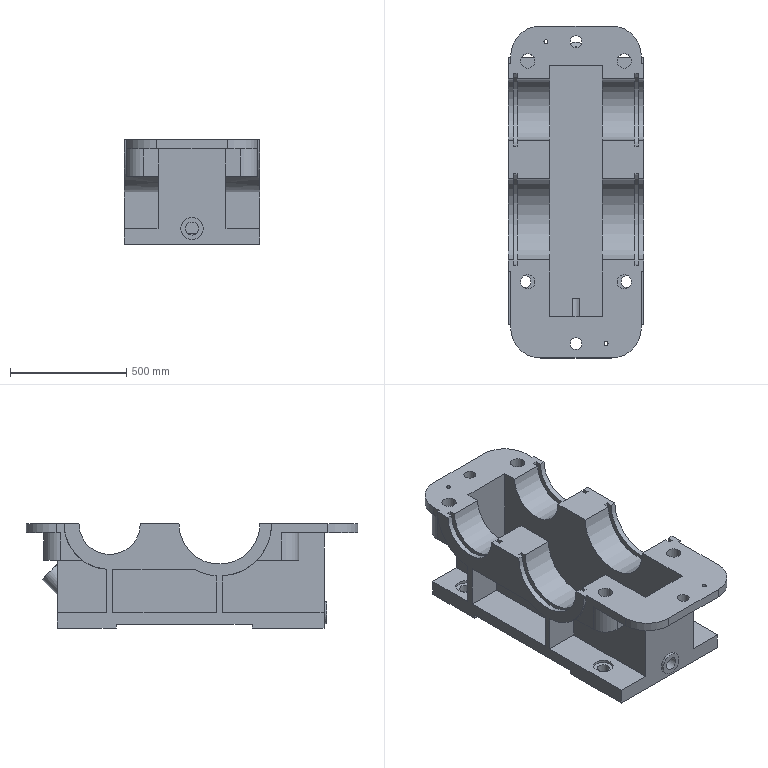Part | NX | features SKETCH 9, BREP 2, DATUM_PLANE 2, SYMBOLIC_THREAD 2, DATUM_CSYS 1, Delete Body 1, LINKED_BODY 1, REPLACE_FACE 1, UNITE 1 | 1 solid | 121 faces | box 585 x 1429 x 450 mm | volume 106130816 mm3 | plane 72 | cylinder 49 | commonest cylinder face diameters 50.625 x6 61.875 x4 84.375 x4 146.25 x4 258.75 x4 264.375 x4